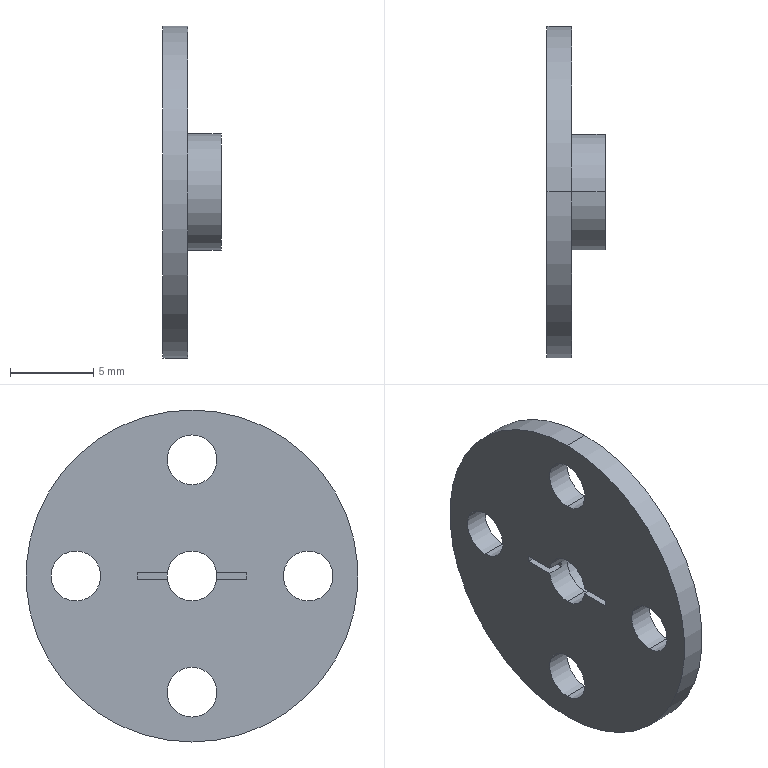Part | STEP file | Large servo disc | 1 solid | 28 faces | box 3.5 x 20 x 20 mm | volume 468.717 mm3 | cylinder 16 | plane 12 | commonest cylinder face diameters 3 x10 4 x2 7 x2 20 x2